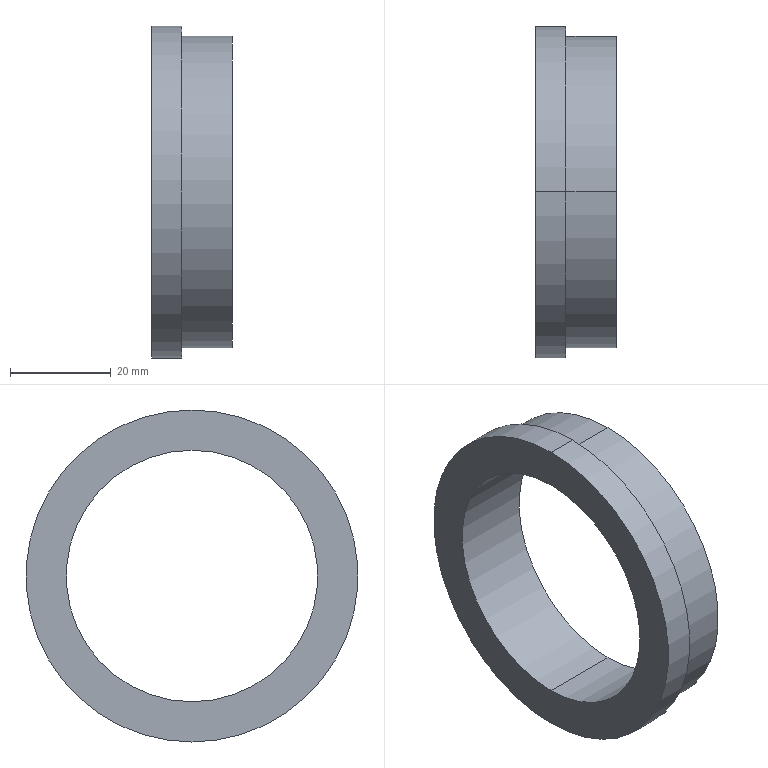Part | SolidWorks | features Revolution 1 | 1 solid | 9 faces | box 16 x 66 x 66 mm | volume 19302 mm3 | cylinder 6 | plane 3 | commonest cylinder face diameters 50 x2 62 x2 66 x2
STEP:
#1=CARTESIAN_POINT('',(6.,0.,33.));
#2=VERTEX_POINT('',#1);
#3=CARTESIAN_POINT('',(6.,0.,-33.));
#4=VERTEX_POINT('',#3);
#5=CARTESIAN_POINT('',(6.,0.,0.));
#6=DIRECTION('',(-1.,0.,0.));
#7=DIRECTION('',(0.,0.,1.));
#8=AXIS2_PLACEMENT_3D('',#5,#6,#7);
#9=CIRCLE('',#8,33.);
#10=EDGE_CURVE('',#2,#4,#9,.T.);
#11=ORIENTED_EDGE('',*,*,#10,.T.);
#12=CARTESIAN_POINT('',(0.,0.,-33.));
#13=VERTEX_POINT('',#12);
#14=CARTESIAN_POINT('',(0.,0.,-33.));
#15=DIRECTION('',(-1.,0.,0.));
#16=VECTOR('',#15,1000.);
#17=LINE('',#14,#16);
#18=EDGE_CURVE('',#4,#13,#17,.T.);
#19=ORIENTED_EDGE('',*,*,#18,.T.);
#20=CARTESIAN_POINT('',(0.,0.,33.));
#21=VERTEX_POINT('',#20);
#22=CARTESIAN_POINT('',(0.,0.,0.));
#23=DIRECTION('',(-1.,0.,0.));
#24=DIRECTION('',(0.,0.,1.));
#25=AXIS2_PLACEMENT_3D('',#22,#23,#24);
#26=CIRCLE('',#25,33.);
#27=EDGE_CURVE('',#21,#13,#26,.T.);
#28=ORIENTED_EDGE('',*,*,#27,.F.);
#29=CARTESIAN_POINT('',(0.,0.,33.));
#30=DIRECTION('',(-1.,0.,0.));
#31=VECTOR('',#30,1000.);
#32=LINE('',#29,#31);
#33=EDGE_CURVE('',#2,#21,#32,.T.);
#34=ORIENTED_EDGE('',*,*,#33,.F.);
#35=EDGE_LOOP('',(#11,#19,#28,#34));
#36=FACE_OUTER_BOUND('',#35,.T.);
#37=CARTESIAN_POINT('',(0.,0.,0.));
#38=DIRECTION('',(-1.,0.,0.));
#39=DIRECTION('',(0.,0.,1.));
#40=AXIS2_PLACEMENT_3D('',#37,#38,#39);
#41=CYLINDRICAL_SURFACE('',#40,33.);
#42=ADVANCED_FACE('',(#36),#41,.T.);
#43=CARTESIAN_POINT('',(16.,0.,31.));
#44=VERTEX_POINT('',#43);
#45=CARTESIAN_POINT('',(16.,0.,-31.));
#46=VERTEX_POINT('',#45);
#47=CARTESIAN_POINT('',(16.,0.,0.));
#48=DIRECTION('',(-1.,0.,0.));
#49=DIRECTION('',(0.,0.,1.));
#50=AXIS2_PLACEMENT_3D('',#47,#48,#49);
#51=CIRCLE('',#50,31.);
#52=EDGE_CURVE('',#44,#46,#51,.T.);
#53=ORIENTED_EDGE('',*,*,#52,.T.);
#54=CARTESIAN_POINT('',(6.,0.,-31.));
#55=VERTEX_POINT('',#54);
#56=CARTESIAN_POINT('',(0.,0.,-31.));
#57=DIRECTION('',(-1.,0.,0.));
#58=VECTOR('',#57,1000.);
#59=LINE('',#56,#58);
#60=EDGE_CURVE('',#46,#55,#59,.T.);
#61=ORIENTED_EDGE('',*,*,#60,.T.);
#62=CARTESIAN_POINT('',(6.,0.,31.));
#63=VERTEX_POINT('',#62);
#64=CARTESIAN_POINT('',(6.,0.,0.));
#65=DIRECTION('',(-1.,0.,0.));
#66=DIRECTION('',(0.,0.,1.));
#67=AXIS2_PLACEMENT_3D('',#64,#65,#66);
#68=CIRCLE('',#67,31.);
#69=EDGE_CURVE('',#63,#55,#68,.T.);
#70=ORIENTED_EDGE('',*,*,#69,.F.);
#71=CARTESIAN_POINT('',(0.,0.,31.));
#72=DIRECTION('',(-1.,0.,0.));
#73=VECTOR('',#72,1000.);
#74=LINE('',#71,#73);
#75=EDGE_CURVE('',#44,#63,#74,.T.);
#76=ORIENTED_EDGE('',*,*,#75,.F.);
#77=EDGE_LOOP('',(#53,#61,#70,#76));
#78=FACE_OUTER_BOUND('',#77,.T.);
#79=CARTESIAN_POINT('',(0.,0.,0.));
#80=DIRECTION('',(-1.,0.,0.));
#81=DIRECTION('',(0.,0.,1.));
#82=AXIS2_PLACEMENT_3D('',#79,#80,#81);
#83=CYLINDRICAL_SURFACE('',#82,31.);
#84=ADVANCED_FACE('',(#78),#83,.T.);
#85=CARTESIAN_POINT('',(16.,0.,-25.));
#86=VERTEX_POINT('',#85);
#87=CARTESIAN_POINT('',(16.,0.,25.));
#88=VERTEX_POINT('',#87);
#89=CARTESIAN_POINT('',(16.,0.,0.));
#90=DIRECTION('',(-1.,0.,0.));
#91=DIRECTION('',(0.,0.,1.));
#92=AXIS2_PLACEMENT_3D('',#89,#90,#91);
#93=CIRCLE('',#92,25.);
#94=EDGE_CURVE('',#86,#88,#93,.T.);
#95=ORIENTED_EDGE('',*,*,#94,.F.);
#96=CARTESIAN_POINT('',(0.,0.,-25.));
#97=VERTEX_POINT('',#96);
#98=CARTESIAN_POINT('',(0.,0.,-25.));
#99=DIRECTION('',(-1.,0.,0.));
#100=VECTOR('',#99,1000.);
#101=LINE('',#98,#100);
#102=EDGE_CURVE('',#86,#97,#101,.T.);
#103=ORIENTED_EDGE('',*,*,#102,.T.);
#104=CARTESIAN_POINT('',(0.,0.,25.));
#105=VERTEX_POINT('',#104);
#106=CARTESIAN_POINT('',(0.,0.,0.));
#107=DIRECTION('',(-1.,0.,0.));
#108=DIRECTION('',(0.,0.,1.));
#109=AXIS2_PLACEMENT_3D('',#106,#107,#108);
#110=CIRCLE('',#109,25.);
#111=EDGE_CURVE('',#97,#105,#110,.T.);
#112=ORIENTED_EDGE('',*,*,#111,.T.);
#113=CARTESIAN_POINT('',(0.,0.,25.));
#114=DIRECTION('',(-1.,0.,0.));
#115=VECTOR('',#114,1000.);
#116=LINE('',#113,#115);
#117=EDGE_CURVE('',#88,#105,#116,.T.);
#118=ORIENTED_EDGE('',*,*,#117,.F.);
#119=EDGE_LOOP('',(#95,#103,#112,#118));
#120=FACE_OUTER_BOUND('',#119,.T.);
#121=CARTESIAN_POINT('',(0.,0.,0.));
#122=DIRECTION('',(-1.,0.,0.));
#123=DIRECTION('',(0.,0.,1.));
#124=AXIS2_PLACEMENT_3D('',#121,#122,#123);
#125=CYLINDRICAL_SURFACE('',#124,25.);
#126=ADVANCED_FACE('',(#120),#125,.F.);
#127=CARTESIAN_POINT('',(0.,0.,0.));
#128=DIRECTION('',(-1.,0.,0.));
#129=DIRECTION('',(0.,0.,1.));
#130=AXIS2_PLACEMENT_3D('',#127,#128,#129);
#131=CIRCLE('',#130,25.);
#132=EDGE_CURVE('',#105,#97,#131,.T.);
#133=ORIENTED_EDGE('',*,*,#132,.F.);
#134=ORIENTED_EDGE('',*,*,#111,.F.);
#135=EDGE_LOOP('',(#133,#134));
#136=FACE_BOUND('',#135,.T.);
#137=ORIENTED_EDGE('',*,*,#27,.T.);
#138=CARTESIAN_POINT('',(0.,0.,0.));
#139=DIRECTION('',(-1.,0.,0.));
#140=DIRECTION('',(0.,0.,1.));
#141=AXIS2_PLACEMENT_3D('',#138,#139,#140);
#142=CIRCLE('',#141,33.);
#143=EDGE_CURVE('',#13,#21,#142,.T.);
#144=ORIENTED_EDGE('',*,*,#143,.T.);
#145=EDGE_LOOP('',(#137,#144));
#146=FACE_OUTER_BOUND('',#145,.T.);
#147=CARTESIAN_POINT('',(0.,33.,0.));
#148=DIRECTION('',(1.,0.,0.));
#149=DIRECTION('',(0.,0.,-1.));
#150=AXIS2_PLACEMENT_3D('',#147,#148,#149);
#151=PLANE('',#150);
#152=ADVANCED_FACE('',(#136,#146),#151,.F.);
#153=ORIENTED_EDGE('',*,*,#102,.F.);
#154=CARTESIAN_POINT('',(16.,0.,0.));
#155=DIRECTION('',(-1.,0.,0.));
#156=DIRECTION('',(0.,0.,1.));
#157=AXIS2_PLACEMENT_3D('',#154,#155,#156);
#158=CIRCLE('',#157,25.);
#159=EDGE_CURVE('',#88,#86,#158,.T.);
#160=ORIENTED_EDGE('',*,*,#159,.F.);
#161=ORIENTED_EDGE('',*,*,#117,.T.);
#162=ORIENTED_EDGE('',*,*,#132,.T.);
#163=EDGE_LOOP('',(#153,#160,#161,#162));
#164=FACE_OUTER_BOUND('',#163,.T.);
#165=CARTESIAN_POINT('',(0.,0.,0.));
#166=DIRECTION('',(-1.,0.,0.));
#167=DIRECTION('',(0.,0.,1.));
#168=AXIS2_PLACEMENT_3D('',#165,#166,#167);
#169=CYLINDRICAL_SURFACE('',#168,25.);
#170=ADVANCED_FACE('',(#164),#169,.F.);
#171=ORIENTED_EDGE('',*,*,#52,.F.);
#172=CARTESIAN_POINT('',(16.,0.,0.));
#173=DIRECTION('',(-1.,0.,0.));
#174=DIRECTION('',(0.,0.,1.));
#175=AXIS2_PLACEMENT_3D('',#172,#173,#174);
#176=CIRCLE('',#175,31.);
#177=EDGE_CURVE('',#46,#44,#176,.T.);
#178=ORIENTED_EDGE('',*,*,#177,.F.);
#179=EDGE_LOOP('',(#171,#178));
#180=FACE_OUTER_BOUND('',#179,.T.);
#181=ORIENTED_EDGE('',*,*,#159,.T.);
#182=ORIENTED_EDGE('',*,*,#94,.T.);
#183=EDGE_LOOP('',(#181,#182));
#184=FACE_BOUND('',#183,.T.);
#185=CARTESIAN_POINT('',(16.,25.,0.));
#186=DIRECTION('',(-1.,0.,0.));
#187=DIRECTION('',(0.,0.,1.));
#188=AXIS2_PLACEMENT_3D('',#185,#186,#187);
#189=PLANE('',#188);
#190=ADVANCED_FACE('',(#180,#184),#189,.F.);
#191=ORIENTED_EDGE('',*,*,#60,.F.);
#192=ORIENTED_EDGE('',*,*,#177,.T.);
#193=ORIENTED_EDGE('',*,*,#75,.T.);
#194=CARTESIAN_POINT('',(6.,0.,0.));
#195=DIRECTION('',(-1.,0.,0.));
#196=DIRECTION('',(0.,0.,1.));
#197=AXIS2_PLACEMENT_3D('',#194,#195,#196);
#198=CIRCLE('',#197,31.);
#199=EDGE_CURVE('',#55,#63,#198,.T.);
#200=ORIENTED_EDGE('',*,*,#199,.F.);
#201=EDGE_LOOP('',(#191,#192,#193,#200));
#202=FACE_OUTER_BOUND('',#201,.T.);
#203=CARTESIAN_POINT('',(0.,0.,0.));
#204=DIRECTION('',(-1.,0.,0.));
#205=DIRECTION('',(0.,0.,1.));
#206=AXIS2_PLACEMENT_3D('',#203,#204,#205);
#207=CYLINDRICAL_SURFACE('',#206,31.);
#208=ADVANCED_FACE('',(#202),#207,.T.);
#209=ORIENTED_EDGE('',*,*,#10,.F.);
#210=CARTESIAN_POINT('',(6.,0.,0.));
#211=DIRECTION('',(-1.,0.,0.));
#212=DIRECTION('',(0.,0.,1.));
#213=AXIS2_PLACEMENT_3D('',#210,#211,#212);
#214=CIRCLE('',#213,33.);
#215=EDGE_CURVE('',#4,#2,#214,.T.);
#216=ORIENTED_EDGE('',*,*,#215,.F.);
#217=EDGE_LOOP('',(#209,#216));
#218=FACE_OUTER_BOUND('',#217,.T.);
#219=ORIENTED_EDGE('',*,*,#69,.T.);
#220=ORIENTED_EDGE('',*,*,#199,.T.);
#221=EDGE_LOOP('',(#219,#220));
#222=FACE_BOUND('',#221,.T.);
#223=CARTESIAN_POINT('',(6.,31.,0.));
#224=DIRECTION('',(-1.,0.,0.));
#225=DIRECTION('',(0.,0.,1.));
#226=AXIS2_PLACEMENT_3D('',#223,#224,#225);
#227=PLANE('',#226);
#228=ADVANCED_FACE('',(#218,#222),#227,.F.);
#229=ORIENTED_EDGE('',*,*,#18,.F.);
#230=ORIENTED_EDGE('',*,*,#215,.T.);
#231=ORIENTED_EDGE('',*,*,#33,.T.);
#232=ORIENTED_EDGE('',*,*,#143,.F.);
#233=EDGE_LOOP('',(#229,#230,#231,#232));
#234=FACE_OUTER_BOUND('',#233,.T.);
#235=CARTESIAN_POINT('',(0.,0.,0.));
#236=DIRECTION('',(-1.,0.,0.));
#237=DIRECTION('',(0.,0.,1.));
#238=AXIS2_PLACEMENT_3D('',#235,#236,#237);
#239=CYLINDRICAL_SURFACE('',#238,33.);
#240=ADVANCED_FACE('',(#234),#239,.T.);
#241=CLOSED_SHELL('',(#42,#84,#126,#152,#170,#190,#208,#228,#240));
#242=MANIFOLD_SOLID_BREP('',#241);
#243=CARTESIAN_POINT('',(0.,0.,0.));
#244=DIRECTION('',(0.,0.,1.));
#245=DIRECTION('',(1.,0.,0.));
#246=AXIS2_PLACEMENT_3D('',#243,#244,#245);
#247=(LENGTH_UNIT()NAMED_UNIT(*)SI_UNIT(.MILLI.,.METRE.));
#248=UNCERTAINTY_MEASURE_WITH_UNIT(LENGTH_MEASURE(0.00001),#247,'','');
#249=(NAMED_UNIT(*)PLANE_ANGLE_UNIT()SI_UNIT($,.RADIAN.));
#250=(NAMED_UNIT(*)SI_UNIT($,.STERADIAN.)SOLID_ANGLE_UNIT());
#251=(GEOMETRIC_REPRESENTATION_CONTEXT(3)GLOBAL_UNCERTAINTY_ASSIGNED_CONTEXT((#248))GLOBAL_UNIT_ASSIGNED_CONTEXT((#247,#249,#250))REPRESENTATION_CONTEXT('',''));
#252=ADVANCED_BREP_SHAPE_REPRESENTATION('',(#242,#246),#251);